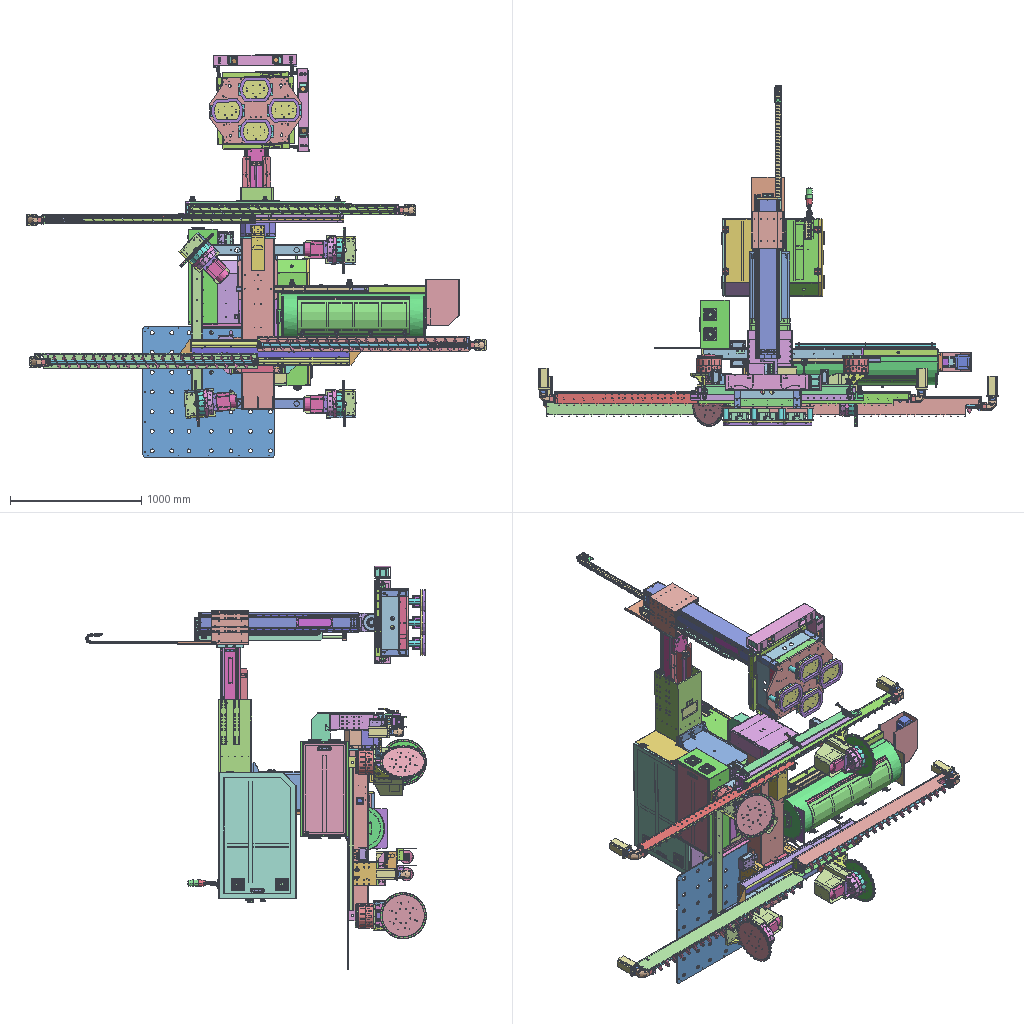Assembly | SolidWorks | 420 different items | 1007 placed | box 3503 x 2594 x 3070 mm
Parts list (item | name | quantity | parent item | size | volume | features), first 271 of 420 items:
1 | 790 Boom +300 Hydraulic Cylinder  (subassembly) | x1 | - | - | - | -
2 | (subassembly) | x4 | in 46 | 270 x 30 x 44 mm | 212143 mm3 | -
3 | (subassembly) | x4 | in 24 | 400 x 30 x 44 mm | 248543 mm3 | -
4 | (subassembly) | x4 | in 19 | 531 x 30 x 44 mm | 286413 mm3 | -
5 | (subassembly) | x2 | in 31 | - | 680804 mm3 | -
6 | (subassembly) | x1 | in 35 | 19.25 x 6.5 x 850 mm | 61984 mm3 | features AEMSimFeature 1
7 | (subassembly) | x2 | in 45 | 80.5 x 70 x 1200 mm | 2951640 mm3 | features ReferencePattern 2, LocalLPattern 1
8 | (subassembly) | x1 | - | - | - | features InContextFeatHolder 31, ReferencePattern 2, AEMSimFeature 1, CenterOfMass 1, LocalLPattern 1
9 | (subassembly) | x1 | - | - | 76260531 mm3 | features CompositeCurve 7
10 | (subassembly) | x1 | in 9 | 250.5 x 328.6 x 299.355 mm | 6826026 mm3 | -
11 | (subassembly) | x1 | in 16 | 1155 x 74 x 49 mm | 647378 mm3 | features AEMSimFeature 1
12 | (subassembly) | x1 | in 9 | 1365 x 260 x 1300 mm | 14682038 mm3 | -
13 | (subassembly) | x1 | - | 375 x 504.5 x 234 mm | 8003020 mm3 | features InContextFeatHolder 28, CompositeCurve 7
14 | (subassembly) | x4 | in 9 | 400 x 532.5 x 350 mm | 11036293 mm3 | features InContextFeatHolder 38, CompositeCurve 7
15 | (subassembly) | x1 | - | - | 69065050 mm3 | features InContextFeatHolder 16
16 | (subassembly) | x1 | - | - | 23045702 mm3 | features InContextFeatHolder 23
17 | (subassembly) | x1 | in 16 | 290 x 578 x 296 mm | 6218838 mm3 | features InContextFeatHolder 10
18 | (subassembly) | x2 | in 15, 16 | 188 x 30 x 80 mm | 347736 mm3 | features InContextFeatHolder 4
19 | (subassembly) | x1 | - | - | 22718189 mm3 | features CompositeCurve 32, InContextFeatHolder 24
20 | (subassembly) | x2 | in 19 | 630 x 120 x 80 mm | 2553807 mm3 | -
21 | (subassembly) | x4 | in 19 | 180 x 166 x 261 mm | 1533619 mm3 | features InContextFeatHolder 4
22 | (subassembly) | x1 | in 15 | 1210 x 74 x 49 mm | 674376 mm3 | features AEMSimFeature 1
23 | (subassembly) | x1 | - | - | 27603448 mm3 | features InContextFeatHolder 30, CenterOfMass 1
24 | (subassembly) | x1 | in 23 | - | 6265247 mm3 | features InContextFeatHolder 2
25 | (subassembly) | x1 | - | 312 x 120 x 1735 mm | 4939212 mm3 | features InContextFeatHolder 4
26 | (subassembly) | x1 | in 23 | 222.5 x 263.631 x 407 mm | 6113754 mm3 | features InContextFeatHolder 12
27 | (subassembly) | x4 | in 23, 49, 50 | 60 x 120 x 112 mm | 205676 mm3 | features InContextFeatHolder 4
28 | (subassembly) | x1 | - | 307 x 120 x 1730 mm | 4796774 mm3 | features InContextFeatHolder 2
29 | (subassembly) | x1 | in 31 | 286 x 85 x 1747 mm | 3475124 mm3 | features InContextFeatHolder 8, CompositeCurve 2
30 | (subassembly) | x1 | in 31 | 286 x 85 x 1747 mm | 3499831 mm3 | features InContextFeatHolder 8
31 | (subassembly) | x1 | in 23 | - | 13765877 mm3 | features InContextFeatHolder 20
32 | (subassembly) | x4 | in 41, 42 | 48 x 11 x 54 mm | 10139 mm3 | -
33 | (subassembly) | x1 | - | 645 x 163.197 x 1205 mm | 2491880 mm3 | features InContextFeatHolder 6
34 | (subassembly) | x1 | - | - | 14201492 mm3 | features InContextFeatHolder 8
35 | (subassembly) | x1 | in 34 | 487 x 297 x 1116 mm | 6337881 mm3 | features ReferencePattern 3, LocalLPattern 1
36 | (subassembly) | x1 | in 34 | 289.417 x 289.417 x 1144 mm | 3340527 mm3 | features ReferencePattern 19, CompositeCurve 2, LocalCirPattern 1
37 | (subassembly) | x1 | - | - | 11450307 mm3 | features ReferencePattern 24, InContextFeatHolder 4, LocalLPattern 3, CompositeCurve 1
38 | (subassembly) | x1 | in 37 | 730 x 365 x 229.027 mm | 2279272 mm3 | -
39 | (subassembly) | x1 | - | 1000 x 8 x 1000 mm | 7675541 mm3 | -
40 | (subassembly) | x1 | - | - | - | features InContextFeatHolder 9
41 | (subassembly) | x1 | in 40 | - | - | features InContextFeatHolder 12
42 | (subassembly) | x1 | in 40 | - | 8213820 mm3 | features InContextFeatHolder 11, ReferencePattern 7, LocalLPattern 1
43 | (subassembly) | x2 | in 15 | 648.543 x 75.872 x 50 mm | 242842 mm3 | features ReferencePattern 15, LocalLPattern 2
44 | (subassembly) | x1 | in 40 | 415.8 x 588 x 32.227 mm | 489087 mm3 | -
45 | (subassembly) | x1 | - | - | 24673962 mm3 | features InContextFeatHolder 11
46 | (subassembly) | x2 | in 45 | - | 3170015 mm3 | features InContextFeatHolder 15, CompositeCurve 2, Belt 1
47 | (subassembly) | x1 | in 45 | 120 x 307 x 1742 mm | 4964407 mm3 | features CompositeCurve 2
48 | (subassembly) | x1 | in 45 | 307 x 120 x 1742 mm | 4354852 mm3 | features CompositeCurve 2
49 | (subassembly) | x1 | - | 120 x 100 x 112 mm | 221397 mm3 | -
50 | (subassembly) | x1 | - | 178.5 x 110 x 112 mm | 250570 mm3 | -
51 | (subassembly) | x3 | in 24, 46 | 20 x 49 x 80 mm | 45972 mm3 | features AEMSimFeature 1
52 | (subassembly) | x3 | in 24, 46 | 44 x 49 x 80 mm | 74061 mm3 | features AEMSimFeature 1
53 | (subassembly) | x2 | in 16 | 960.543 x 75.872 x 50 mm | 342604 mm3 | features ReferencePattern 28, LocalLPattern 2
54 | (subassembly) | x8 | in 31, 35 | 97.135 x 31.44 x 28.2 mm | 12763 mm3 | -
55 | (subassembly) | x7 | in 9, 31 | 161.788 x 44.909 x 44.4 mm | 32694 mm3 | -
56 | (subassembly) | x1 | - | 112 x 125 x 1730 mm | 1536921 mm3 | features ReferencePattern 14, InContextFeatHolder 6, LocalLPattern 2
57 | (subassembly) | x1 | - | 127 x 125 x 1722 mm | 4062488 mm3 | -
58 | (subassembly) | x1 | - | 122 x 130 x 1720 mm | 4058025 mm3 | -
59 | (subassembly) | x1 | - | 246.625 x 216.5 x 351 mm | 5460860 mm3 | features InContextFeatHolder 2, CompositeCurve 1
60 | (subassembly) | x1 | - | 219.765 x 289 x 182 mm | 3217706 mm3 | features InContextFeatHolder 6, CompositeCurve 2
61 | (subassembly) | x1 | - | 490 x 459 x 291.379 mm | 615629 mm3 | features InContextFeatHolder 6
62 | (subassembly) | x3 | in 44 | 14.65 x 4.3 x 40 mm | 1347 mm3 | -
63 | (subassembly) | x1 | - | 150 x 131 x 2150 mm | 4854197 mm3 | -
64 | (subassembly) | x4 | in 37 | 37.408 x 96.6 x 96.6 mm | 223267 mm3 | -
65 | (subassembly) | x1 | - | 1365 x 969.6 x 1300 mm | 30670521 mm3 | features CompositeCurve 17, InContextFeatHolder 10
66 | (subassembly) | x4 | in 16 | 1215 x 30 x 44 mm | 550817 mm3 | -
67 | (subassembly) | x4 | in 15 | - | 682203 mm3 | -
68 | - | x2 | in 41 | 30 x 60 x 830 mm | 242360 mm3 | features Extrusion 1, Shell 1
69 | - | x2 | in 15 | 60 x 60 x 1234 mm | 431666 mm3 | features HoleWzd 4, Chamfer 1, Extrusion 1
70 | - | x8 | in 15, 16 | 81 x 20 x 12 mm | 16180 mm3 | features Chamfer 1, Extrusion 1, HoleWzd 1
71 | - | x1 | in 15 | 170 x 1.5 x 100 mm | 25318 mm3 | features BreakCorner 1, FlatPattern 1, HoleWzd 1, SMBaseFlange 1, SheetMetal 1
72 | - | x4 | in 15 | 20 x 220 x 35 mm | 142848 mm3 | features HoleWzd 2, Chamfer 1, Extrusion 1
73 | - | x4 | in 15 | 20 x 568 x 30 mm | 116464 mm3 | features HoleWzd 2, ICE 1, WeldMemberFeat 1, WeldmentFeature 1
74 | - | x2 | in 15 | 20 x 20 x 354 mm | 109668 mm3 | features HoleWzd 2, Chamfer 1, Extrusion 1
75 | - | x2 | in 15 | 50 x 50 x 650 mm | 247288 mm3 | features Chamfer 1, Extrusion 1, HoleWzd 1
76 | - | x1 | in 15 | 250 x 60 x 1 mm | 14915 mm3 | features BreakCorner 1, FlatPattern 1, HoleWzd 1, SMBaseFlange 1, SheetMetal 1
77 | - | x1 | in 16 | 250 x 250 x 280 mm | 2610401 mm3 | features HoleWzd 8, Chamfer 1, Cut 1, Extrusion 1, MirrorPattern 1
78 | - | x1 | in 16 | 150 x 150 x 1215 mm | 6013792 mm3 | features HoleWzd 14, ICE 3, Cut 2, Fillet 2, Extrusion 1
79 | - | x3 | in 17 | 62 x 138 x 138 mm | 462395 mm3 | features BaseBody 1
80 | - | x1 | in 16 | 84 x 70 x 50 mm | 186072 mm3 | features ICE 5, Chamfer 2, HoleWzd 2, Extrusion 1
81 | - | x4 | in 16 | 47 x 14 x 280 mm | 149226 mm3 | features HoleWzd 2, Chamfer 1, Extrusion 1, MoveFace 1
82 | - | x1 | in 16 | 70 x 278 x 1 mm | 19366 mm3 | features BreakCorner 1, FlatPattern 1, HoleWzd 1, SMBaseFlange 1, SheetMetal 1
83 | - | x2 | in 16 | 60 x 60 x 945 mm | 330466 mm3 | features HoleWzd 2, Chamfer 1, Extrusion 1
84 | - | x1 | in 16 | 257 x 300 x 20 mm | 215937 mm3 | features HoleWzd 2, BreakCorner 1, Chamfer 1, EdgeFlange 1, Extrusion 1, FlatPattern 1, SheetMetal 1, SolidToSheetMetal 1
85 | - | x1 | in 17 | 130 x 12 x 130 mm | 148815 mm3 | features HoleWzd 6, ICE 2, Chamfer 1, Cut 1, Extrusion 1
86 | - | x1 | in 17 | 130 x 12 x 130 mm | 79357 mm3 | features HoleWzd 5, Chamfer 1, Extrusion 1, ICE 1
87 | - | x1 | in 17 | 140 x 165 x 130 mm | 629581 mm3 | features HoleWzd 5, ICE 4, Chamfer 1, Extrusion 1
88 | - | x1 | in 17 | 140 x 165 x 120 mm | 582879 mm3 | features ICE 5, HoleWzd 3, Chamfer 2, Extrusion 1
89 | - | x1 | in 17 | 120 x 136 x 68 mm | 368287 mm3 | features HoleWzd 4, Chamfer 1, Extrusion 1, ICE 1
90 | - | x10 | - | 15.114 x 19.643 x 23.399 mm | 1126 mm3 | features BaseBody 1
91 | - | x1 | in 17 | 120 x 160 x 74 mm | 438042 mm3 | features HoleWzd 4, Chamfer 1, Extrusion 1, ICE 1
92 | - | x2 | in 18 | 188 x 23 x 80 mm | 151717 mm3 | features Fillet 3, HoleWzd 2, ICE 2, Chamfer 1, Extrusion 1
93 | - | x2 | in 18 | 188 x 7 x 80 mm | 69688 mm3 | features HoleWzd 2, Chamfer 1, Extrusion 1, Fillet 1
94 | - | x1 | in 19 | 700 x 15 x 500 mm | 4450228 mm3 | features HoleWzd 5, Cut 1, Extrusion 1, Fillet 1, ICE 1
95 | - | x4 | in 19 | 50 x 260 x 50 mm | 74530 mm3 | features HoleWzd 6, CirPattern 1, Extrusion 1
96 | - | x4 | in 19 | 40 x 50 x 506 mm | 247347 mm3 | features HoleWzd 4, ExtruThin 1
97 | - | x4 | in 19 | 29 x 25 x 40 mm | 10588 mm3 | features HoleWzd 2, Chamfer 1, Extrusion 1
98 | - | x2 | in 19 | 499 x 60 x 10 mm | 297280 mm3 | features HoleWzd 3, Extrusion 1
99 | - | x2 | in 19 | 479 x 60 x 10 mm | 285459 mm3 | features HoleWzd 3, Extrusion 1
100 | - | x4 | in 19 | 496 x 185 x 10 mm | 92290 mm3 | features Cut 2, HoleWzd 2, BreakCorner 1, EdgeFlange 1, FlatPattern 1, ICE 1, SMBaseFlange 1, SheetMetal 1
101 | - | x52 | - | 15.114 x 19.643 x 23.399 mm | 1126 mm3 | features BaseBody 1
102 | - | x2 | in 20 | 80 x 120 x 630 mm | 467928 mm3 | features HoleWzd 2, Cut 1, ExtruThin 1, Fillet 1, ICE 1
103 | - | x4 | in 21 | 180 x 15 x 240 mm | 528961 mm3 | features HoleWzd 4, Extrusion 1, Fillet 1, ICE 1
104 | - | x8 | in 21 | 12 x 63 x 80 mm | 50248 mm3 | features HoleWzd 7, Extrusion 1
105 | - | x4 | in 21 | 83 x 64 x 140 mm | 28826 mm3 | features HoleWzd 2, FlatPattern 1, SMBaseFlange 1, SheetMetal 1
106 | - | x4 | in 21 | 75 x 32 x 70 mm | 77130 mm3 | features HoleWzd 2, ICE 2, Extrusion 1
107 | - | x4 | in 21 | 75 x 58 x 3 mm | 8829 mm3 | features ICE 2, Extrusion 1, Fillet 1, HoleWzd 1
108 | - | x4 | in 21 | 75 x 29 x 40 mm | 38371 mm3 | features Extrusion 1, HoleWzd 1, ICE 1, MoveFace 1
109 | - | x4 | in 21 | 54.631 x 35.5 x 20 mm | 24661 mm3 | features ICE 3, Extrusion 1, Fillet 1, HoleWzd 1
110 | - | x2 | in 23 | 40 x 80 x 60 mm | 12649 mm3 | features HoleWzd 2, BreakCorner 1, FlatPattern 1, SMBaseFlange 1, SheetMetal 1
111 | - | x1 | in 24 | 250 x 400 x 100 mm | 1758243 mm3 | features HoleWzd 10, Fillet 3, ICE 3, Cut 2, Extrusion 1, MirrorPattern 1
112 | - | x1 | in 24 | 60 x 135 x 60 mm | 337667 mm3 | features BaseBody 1
113 | - | x1 | in 24 | 12 x 345 x 110 mm | 373766 mm3 | features HoleWzd 4, Cut 1, Extrusion 1
114 | - | x1 | in 24 | 12 x 345 x 110 mm | 373766 mm3 | features HoleWzd 4, Cut 1, Extrusion 1
115 | - | x1 | in 24 | 10 x 330 x 180 mm | 549177 mm3 | features Cut 2, HoleWzd 2, Chamfer 1, Extrusion 1, MoveFace 1
116 | - | x1 | in 24 | 55 x 65.5 x 30 mm | 74891 mm3 | features HoleWzd 3, Chamfer 2, ICE 2, Extrusion 1
117 | - | x4 | in 24 | 35 x 12 x 16 mm | 5336 mm3 | features Chamfer 1, Extrusion 1, HoleWzd 1
118 | - | x1 | in 24 | 100 x 60 x 110 mm | 155366 mm3 | features Chamfer 2, HoleWzd 2, Extrusion 1, MoveFace 1
119 | - | x1 | in 24 | 347 x 403 x 127.5 mm | 464397 mm3 | features HoleWzd 3, ICE 3, Cut 2, FlatPattern 2, SheetMetal 2, SolidToSheetMetal 2, BreakCorner 1, Chamfer 1, EdgeFlange 1, Extrusion 1, MirrorPattern 1
120 | - | x1 | in 24 | 260 x 145 x 128 mm | 125858 mm3 | features Chamfer 2, EdgeFlange 2, Extrusion 1, FlatPattern 1, HoleWzd 1, SheetMetal 1, SolidToSheetMetal 1
121 | - | x1 | in 24 | 250 x 1.5 x 100 mm | 37100 mm3 | features BreakCorner 1, FlatPattern 1, HoleWzd 1, ICE 1, SMBaseFlange 1, SheetMetal 1
122 | - | x1 | in 24 | 104 x 10 x 60 mm | 39122 mm3 | features HoleWzd 4, Cut 2, Chamfer 1, Extrusion 1
123 | - | x2 | in 34 | 55 x 55 x 13 mm | 21668 mm3 | features Extrusion 1, Fillet 1
124 | - | x1 | in 24 | 70 x 10 x 60 mm | 36663 mm3 | features HoleWzd 4, Chamfer 1, Extrusion 1
125 | - | x2 | in 24 | 40 x 30 x 8 mm | 6006 mm3 | features Chamfer 1, Extrusion 1, HoleWzd 1
126 | - | x1 | in 24 | 100 x 60 x 110 mm | 155366 mm3 | features Chamfer 2, HoleWzd 2, Extrusion 1, MoveFace 1
127 | - | x1 | - | 120 x 75 x 1000 mm | 1739267 mm3 | features HoleWzd 5, Cut 2, MoveFace 2, Chamfer 1, Extrusion 1, Fillet 1
128 | - | x2 | in 47, 48 | 100 x 100 x 1604 mm | 874347 mm3 | features MoveFace 6, ICE 2, BaseBody 1, Helix 1, Sweep 1
129 | - | x2 | in 47, 48 | 50 x 50 x 10 mm | 11856 mm3 | features ICE 2, Chamfer 1, Extrusion 1, HoleWzd 1
130 | - | x4 | in 29, 30, 47, 48 | 50 x 50 x 10 mm | 10238 mm3 | features ICE 2, Chamfer 1, Extrusion 1, HoleWzd 1
131 | - | x4 | in 29, 30, 47, 48 | 62 x 62 x 12 mm | 24839 mm3 | features ICE 3, HoleWzd 2, Chamfer 1, Extrusion 1
132 | - | x1 | in 47 | 92 x 99 x 15 mm | 82233 mm3 | features MirrorStock 1
133 | - | x1 | in 47 | 87 x 94 x 12 mm | 62817 mm3 | features MirrorStock 1
134 | - | x10 | in 15, 16, 17, 26, 29, 30, 47, 48 | 180 x 81 x 81 mm | 861564 mm3 | features BaseBody 1, MoveFace 1
135 | - | x4 | in 29, 30, 47, 48 | 85 x 13 x 85 mm | 56434 mm3 | features ICE 3, HoleWzd 2, Chamfer 1, Extrusion 1
136 | - | x1 | - | 150 x 120 x 1609 mm | 2357171 mm3 | features HoleWzd 7, Fillet 2, Cut 1, Extrusion 1, ICE 1, LPattern 1, MoveFace 1
137 | - | x1 | in 48 | 87 x 94 x 12 mm | 62817 mm3 | features HoleWzd 4, Cut 2, MoveFace 2, Chamfer 1, Extrusion 1, Fillet 1, ICE 1
138 | - | x1 | in 48 | 92 x 99 x 15 mm | 82233 mm3 | features HoleWzd 4, Cut 2, MoveFace 2, Chamfer 1, Extrusion 1, Fillet 1, ICE 1, MoveCopyBody 1
139 | - | x1 | in 26 | 260 x 260 x 20 mm | 876981 mm3 | features HoleWzd 6, Chamfer 3, ICE 2, Extrusion 1, Fillet 1
140 | - | x1 | in 26 | 100 x 17.5 x 100 mm | 79036 mm3 | features ICE 6, HoleWzd 4, Chamfer 3, Extrusion 1, Fillet 1
141 | - | x1 | in 26 | 262.631 x 60 x 222.5 mm | 1391855 mm3 | features HoleWzd 5, ICE 5, Chamfer 1, Cut 1, Fillet 1, Revolution 1
142 | - | x1 | in 26 | 44 x 47.656 x 48 mm | 38750 mm3 | features ICE 5, HoleWzd 4, BaseBody 1, Chamfer 1, RevCut 1
143 | - | x1 | in 26 | 263 x 130.5 x 136 mm | 76891 mm3 | features HoleWzd 2, Chamfer 1, Cut 1, Extrusion 1, Shell 1
144 | - | x1 | in 26 | 263 x 130.5 x 136 mm | 68260 mm3 | features Cut 2, HoleWzd 2, Chamfer 1, Extrusion 1, Shell 1
145 | - | x1 | in 41 | 110 x 15 x 20 mm | 32457 mm3 | features Extrusion 1, HoleWzd 1
146 | - | x1 | in 26 | 340 x 95 x 103 mm | 87299 mm3 | features EdgeFlange 1, Extrusion 1, FlatPattern 1, HoleWzd 1, ICE 1, SheetMetal 1, SolidToSheetMetal 1
147 | - | x4 | in 27 | 60 x 120 x 90 mm | 122991 mm3 | features HoleWzd 4, Extrusion 1, Shell 1
148 | - | x4 | in 27 | 60 x 120 x 4 mm | 27931 mm3 | features Extrusion 1, HoleWzd 1, ICE 1
149 | - | x4 | in 27 | 60 x 120 x 4 mm | 16436 mm3 | features HoleWzd 4, ICE 3, Extrusion 1, Fillet 1
150 | - | x4 | in 27 | 50 x 110 x 2 mm | 11000 mm3 | features Extrusion 1
151 | - | x1 | in 31 | 150 x 105 x 1200 mm | 2927452 mm3 | features HoleWzd 7, Extrusion 1, MoveFace 1
152 | - | x1 | in 31 | 120 x 75 x 1150 mm | 2118632 mm3 | features HoleWzd 4, Extrusion 1
153 | - | x2 | in 31 | 70 x 50 x 60 mm | 59657 mm3 | features HoleWzd 2, Chamfer 1, Extrusion 1
154 | - | x1 | in 31 | 80 x 99 x 60 mm | 93057 mm3 | features HoleWzd 2, Chamfer 1, Extrusion 1
155 | - | x1 | in 31 | 80 x 22 x 60 mm | 46558 mm3 | features HoleWzd 2, Chamfer 1, Extrusion 1
156 | - | x2 | in 15, 16 | 90.001 x 150.5 x 90.001 mm | 719392 mm3 | features BaseBody 1
157 | - | x1 | in 30 | 110 x 70 x 1620 mm | 1292912 mm3 | features HoleWzd 8, Extrusion 1, Fillet 1, ICE 1, LPattern 1
158 | - | x2 | in 29, 30 | 60 x 60 x 1608 mm | 669681 mm3 | features MoveFace 7, ICE 2, BaseBody 1, Helix 1, Sweep 1
159 | - | x2 | in 29, 30 | 50 x 50 x 10 mm | 15222 mm3 | features ICE 2, Chamfer 1, Extrusion 1, HoleWzd 1
160 | - | x1 | in 30 | 65 x 81 x 15 mm | 49071 mm3 | features HoleWzd 2, MoveFace 2, MirrorStock 1
161 | - | x1 | in 30 | 60 x 76 x 12 mm | 39739 mm3 | features HoleWzd 2, MoveFace 2, MirrorStock 1
162 | - | x1 | in 29 | 110 x 70 x 1620 mm | 1267846 mm3 | features HoleWzd 8, MoveFace 3, Fillet 2, LPattern 2, Cut 1, Extrusion 1, ICE 1
163 | - | x1 | in 29 | 65 x 81 x 15 mm | 49071 mm3 | features HoleWzd 4, Cut 2, MoveFace 2, Chamfer 1, Extrusion 1, Fillet 1, ICE 1, MoveCopyBody 1
164 | - | x1 | in 29 | 60 x 76 x 12 mm | 39739 mm3 | features HoleWzd 4, MoveFace 3, Cut 2, Chamfer 1, Extrusion 1, Fillet 1, ICE 1
165 | - | x1 | in 34 | 142 x 173 x 34 mm | 50656 mm3 | features EdgeFlange 2, HoleWzd 2, BreakCorner 1, FlatPattern 1, MoveFace 1, SMBaseFlange 1, SheetMetal 1
166 | - | x8 | in 41, 42, 64 | 92 x 92.001 x 25.408 mm | 167387 mm3 | features BaseBody 1
167 | - | x1 | in 34 | 187 x 372 x 254 mm | 400780 mm3 | features FlatPattern 2, SheetMetal 2, BreakCorner 1, Chamfer 1, Extrusion 1, HoleWzd 1, SMBaseFlange 1, SolidToSheetMetal 1
168 | - | x1 | in 34 | 110 x 110 x 16 mm | 113885 mm3 | features ICE 3, Chamfer 2, HoleWzd 2, Extrusion 1
169 | - | x1 | in 34 | 100 x 100 x 15 mm | 98385 mm3 | features HoleWzd 2, ICE 2, Chamfer 1, Extrusion 1
170 | - | x1 | in 34 | 140 x 140 x 24 mm | 366967 mm3 | features HoleWzd 3, ICE 3, Chamfer 1, Cut 1, Extrusion 1
171 | - | x1 | in 35 | 487 x 297 x 1116 mm | 5128142 mm3 | features ICE 12, HoleWzd 7, Fillet 4, MoveCopyBody 4, Chamfer 3, LPattern 3, Stock 3, Cut 1, Extrusion 1, Shell 1
172 | - | x1 | in 35 | 284.209 x 71.481 x 850 mm | 1096694 mm3 | features ExtruThin 1, ICE 1
173 | - | x1 | in 36 | 60 x 60 x 92 mm | 149406 mm3 | features ICE 6, Chamfer 1, Extrusion 1, HoleWzd 1
174 | - | x1 | in 36 | 291 x 291 x 5 mm | 156823 mm3 | features ICE 2, Extrusion 1, Fillet 1
175 | - | x2 | in 36 | 291 x 291 x 5 mm | 163158 mm3 | features ICE 2, Extrusion 1, Fillet 1
176 | - | x1 | in 36 | 1022 x 30 x 30 mm | 722056 mm3 | features ICE 3, WeldMemberFeat 1, WeldmentFeature 1
177 | - | x8 | in 14 | 65 x 65 x 7 mm | 9271 mm3 | features BaseBody 1
178 | - | x1 | in 36 | 60 x 60 x 90 mm | 128146 mm3 | features ICE 8, HoleWzd 2, Chamfer 1, Extrusion 1
179 | - | x20 | in 36 | 1072 x 25 x 3 mm | 80400 mm3 | features FlatPattern 1, SMBaseFlange 1, SheetMetal 1
180 | - | x1 | in 36 | 181 x 462.5 x 181 mm | 124893 mm3 | features Helix 1, Sweep 1
181 | - | x1 | in 36 | 181 x 462.5 x 181 mm | 124893 mm3 | features Helix 1, Sweep 1
182 | - | x1 | in 38 | 730 x 365 x 221.5 mm | 1200734 mm3 | features HoleWzd 6, ICE 4, EdgeFlange 3, FlatPattern 1, SheetMetal 1, SolidToSheetMetal 1
183 | - | x1 | in 38 | 693 x 342.263 x 15 mm | 608896 mm3 | features EdgeFlange 3, FlatPattern 2, ICE 2, MoveCopyBody 2, SMBaseFlange 2, SheetMetal 2, Chamfer 1, Cut 1, HoleWzd 1, Stock 1
184 | - | x1 | in 38 | 660 x 305 x 12 mm | 436518 mm3 | features HoleWzd 2, EdgeFlange 1, FlatPattern 1, SMBaseFlange 1, SheetMetal 1
185 | - | x1 | in 39 | 1000 x 8 x 1000 mm | 7675541 mm3 | features HoleWzd 2, MoveFace 2, Cut 1, Extrusion 1, Fillet 1, ICE 1, LPattern 1
186 | - | x2 | in 40 | 20 x 90.5 x 416.5 mm | 94970 mm3 | features EdgeFlange 2, FlatPattern 1, HoleWzd 1, ICE 1, SMBaseFlange 1, SheetMetal 1
187 | - | x1 | in 40 | 298 x 21.5 x 551.5 mm | 305724 mm3 | features EdgeFlange 2, Cut 1, FlatPattern 1, HoleWzd 1, SMBaseFlange 1, SheetMetal 1
188 | - | x4 | in 29, 30, 47, 48 | 35 x 35 x 10 mm | 5588 mm3 | features BaseBody 1
189 | - | x1 | in 40 | 20 x 140 x 90 mm | 21403 mm3 | features HoleWzd 2, BreakCorner 1, FlatPattern 1, SMBaseFlange 1, SheetMetal 1
190 | - | x1 | in 41 | 264.5 x 588 x 960 mm | 1725944 mm3 | features HoleWzd 16, ICE 8, Cut 6, FlatPattern 6, SheetMetal 6, SolidToSheetMetal 4, SMBaseFlange 3, EdgeFlange 2, MoveFace 2, Chamfer 1, Extrusion 1
191 | - | x1 | in 41 | 959 x 587 x 21.5 mm | 1078977 mm3 | features EdgeFlange 4, FlatPattern 4, SMBaseFlange 4, SheetMetal 4, HoleWzd 3, Cut 2, ICE 1
192 | - | x1 | in 41 | 830 x 530 x 15 mm | 919562 mm3 | features HoleWzd 2, BreakCorner 1, Cut 1, EdgeFlange 1, FlatPattern 1, SMBaseFlange 1, SheetMetal 1
193 | - | x1 | in 42 | 233 x 588 x 960 mm | 1652161 mm3 | features HoleWzd 15, FlatPattern 7, ICE 7, SheetMetal 7, SolidToSheetMetal 6, Cut 5, EdgeFlange 3, Chamfer 1, Extrusion 1, SMBaseFlange 1
194 | - | x1 | in 42 | 959 x 587 x 21.5 mm | 1078977 mm3 | features MirrorStock 1
195 | - | x1 | in 42 | 830 x 530 x 15 mm | 919972 mm3 | features HoleWzd 1, ICE 1, MirrorStock 1
196 | - | x1 | in 44 | 16 x 588 x 411.5 mm | 451920 mm3 | features EdgeFlange 2, Cut 1, FlatPattern 1, HoleWzd 1, SMBaseFlange 1, SheetMetal 1
197 | - | x2 | in 45 | 120 x 86 x 195 mm | 136249 mm3 | features HoleWzd 2, BreakCorner 1, Cut 1, EdgeFlange 1, ExtruThin 1, FlatPattern 1, SheetMetal 1, SolidToSheetMetal 1
198 | - | x1 | in 45 | 1200 x 80 x 25 mm | 115619 mm3 | features MoveFace 2, BreakCorner 1, Cut 1, EdgeFlange 1, FlatPattern 1, HoleWzd 1, SMBaseFlange 1, SheetMetal 1
199 | - | x4 | in 29, 30, 47, 48 | 47 x 47 x 12 mm | 12629 mm3 | features BaseBody 1
200 | - | x1 | in 45 | 1200 x 80 x 25 mm | 115619 mm3 | features MirrorStock 1
201 | - | x2 | in 45 | 249 x 116 x 90 mm | 48716 mm3 | features EdgeFlange 2, BreakCorner 1, FlatPattern 1, HoleWzd 1, ICE 1, MoveFace 1, SMBaseFlange 1, SheetMetal 1
202 | - | x1 | in 45 | 195 x 12 x 1200 mm | 2789805 mm3 | features HoleWzd 6, Extrusion 1, ICE 1
203 | - | x1 | in 45 | 90 x 60 x 255 mm | 315166 mm3 | features Chamfer 3, HoleWzd 2, ExtruThin 1
204 | - | x1 | in 45 | 90 x 60 x 255 mm | 315166 mm3 | features MirrorStock 1
205 | - | x2 | in 46 | 180 x 270 x 36 mm | 970158 mm3 | features HoleWzd 11, ICE 2, Cut 1, Extrusion 1, Fillet 1
206 | - | x2 | in 46 | 75 x 39.5 x 34 mm | 65045 mm3 | features HoleWzd 3, Chamfer 2, ICE 2, Extrusion 1
207 | - | x2 | in 46 | 175 x 275 x 15 mm | 588428 mm3 | features HoleWzd 4, Extrusion 1, ICE 1
208 | - | x2 | in 46 | 160 x 8 x 82 mm | 66317 mm3 | features HoleWzd 2, Extrusion 1, Fillet 1, ICE 1
209 | - | x2 | in 46 | 105 x 30 x 120 mm | 37376 mm3 | features HoleWzd 2, BreakCorner 1, Cut 1, Extrusion 1, FlatPattern 1, ICE 1, SheetMetal 1, SolidToSheetMetal 1
210 | - | x2 | in 46 | 184 x 270 x 86 mm | 96917 mm3 | features HoleWzd 2, Extrusion 1, ICE 1, Shell 1
211 | - | x1 | in 47 | 150 x 120 x 1700 mm | 2499600 mm3 | features HoleWzd 10, Fillet 2, LPattern 2, Cut 1, Extrusion 1, ICE 1, MoveFace 1
212 | - | x1 | in 48 | 150 x 120 x 1609 mm | 2345426 mm3 | features HoleWzd 7, Fillet 2, LPattern 2, Cut 1, Extrusion 1, ICE 1, MoveFace 1
213 | - | x4 | in 29, 47, 48 | 50 x 50 x 6 mm | 13563 mm3 | features ICE 3, Chamfer 1, Extrusion 1, HoleWzd 1
214 | - | x1 | in 49 | 40 x 80 x 60 mm | 15721 mm3 | features HoleWzd 2, BreakCorner 1, FlatPattern 1, SMBaseFlange 1, SheetMetal 1
215 | - | x1 | in 50 | 50 x 170 x 70 mm | 44894 mm3 | features HoleWzd 2, BreakCorner 1, FlatPattern 1, Gusset 1, SMBaseFlange 1, SheetMetal 1
216 | - | x2 | in 46 | 46.2 x 152.2 x 15 mm | 20675 mm3 | features BeltProfileFeature 1, ExtruThin 1
217 | - | x1 | in 10 | 250.5 x 250.5 x 122.6 mm | 3466893 mm3 | features BaseBody 1
218 | - | x2 | in 15, 16 | 26 x 60 x 88 mm | 94371 mm3 | features BaseBody 3
219 | - | x4 | in 20 | 196.4 x 105.4 x 59 mm | 1042939 mm3 | features BaseBody 3
220 | - | x2 | in 46 | 21 x 44 x 44 mm | 20059 mm3 | features BaseBody 1
221 | - | x2 | in 46 | 21 x 44 x 44 mm | 16333 mm3 | features BaseBody 1
222 | - | x1 | in 19 | 146.9 x 109.2 x 38 mm | 517225 mm3 | features BaseBody 9
223 | - | x4 | in 14 | 130 x 170 x 202 mm | 1970646 mm3 | features ICE 11, Chamfer 2, Fillet 2, HoleWzd 2, Extrusion 1
224 | - | x3 | in 37 | 50 x 210 x 100 mm | 965694 mm3 | features HoleWzd 2, Extrusion 1, ICE 1
225 | - | x6 | in 14, 46 | 92.5 x 148 x 80 mm | 645645 mm3 | features BaseBody 6
226 | - | x2 | in 15, 16 | 69 x 60 x 88 mm | 168819 mm3 | features BaseBody 9
227 | - | x4 | in 38, 41, 42, 44 | 59.2 x 32.227 x 110 mm | 33125 mm3 | features BaseBody 1
228 | - | x1 | in 19 | 145 x 40 x 90 mm | 467276 mm3 | features Extrusion 1, HoleWzd 1, ICE 1
229 | - | x1 | in 41 | 65 x 79.307 x 65.435 mm | 93271 mm3 | features BaseBody 13
230 | - | x1 | in 41 | - | - | features BaseBody 25, RefSurface 9
231 | - | x1 | in 41 | 70 x 236.301 x 70 mm | 289384 mm3 | features BaseBody 9
232 | - | x8 | in 41, 42, 64 | 96.6 x 96.6 x 10.5 mm | 55881 mm3 | features BaseBody 3
233 | - | x1 | in 41 | 45 x 64 x 90 mm | 259200 mm3 | features Extrusion 1
234 | - | x5 | in 24, 29, 30, 47, 48 | 105 x 143.9 x 60 mm | 435944 mm3 | features BaseBody 10
235 | - | x1 | in 34 | 247 x 90 x 141 mm | 1704334 mm3 | features BaseBody 30
236 | - | x1 | in 26 | 85 x 85 x 145.3 mm | 617481 mm3 | features BaseBody 3
237 | - | x1 | in 41 | - | 778602 mm3 | features BaseBody 96
238 | - | x4 | in 46 | 49 x 11.547 x 10 mm | 1608 mm3 | features RevCut 3, Boss 1, Chamfer 1, Extrusion 1, Fillet 1, LPattern 1
239 | - | x4 | in 46 | 11.547 x 10 x 6.4 mm | 424.571 mm3 | features RevCut 2, Extrusion 1, LPattern 1
240 | - | x1 | in 19 | 70 x 23 x 118 mm | 188768 mm3 | features Extrusion 1, Fillet 1, HoleWzd 1
241 | - | x6 | in 14, 34, 45 | 14.4 x 14 x 14 mm | 897.239 mm3 | features Cut 2, RevCut 2, Boss 1, Extrusion 1, Fillet 1, LPattern 1
242 | - | x8 | in 14, 45, 46 | 51 x 10 x 10 mm | 1665 mm3 | features Fillet 2, RevCut 2, Boss 1, Chamfer 1, Cut 1, Extrusion 1, LPattern 1
243 | - | x1 | in 19 | 64 x 23 x 45 mm | 65028 mm3 | features Extrusion 1, Fillet 1, HoleWzd 1
244 | - | x1 | in 10 | 100 x 10 x 100 mm | 28032 mm3 | features Extrusion 1, Fillet 1
245 | - | x12 | in 18 | 44 x 7 x 44 mm | 4885 mm3 | features Extrusion 1, ICE 1
246 | - | x1 | - | 70 x 200 x 120 mm | 169957 mm3 | features HoleWzd 2, Cut 1, Extrusion 1, ICE 1
247 | - | x8 | in 21 | 88 x 131 x 55 mm | 138232 mm3 | features ICE 2, Extrusion 1, HoleWzd 1
248 | - | x1 | in 24 | 66 x 40 x 40 mm | 67909 mm3 | features BaseBody 3
249 | - | x4 | in 21 | 180 x 20 x 240 mm | 299340 mm3 | features Extrusion 1, Fillet 1
250 | - | x1 | in 41 | 170 x 40 x 180 mm | 1224000 mm3 | features Extrusion 1
251 | - | x1 | - | 60 x 60 x 60 mm | 25462 mm3 | features HoleWzd 2, Chamfer 1, Extrusion 1
252 | - | x1 | - | 70 x 200 x 120 mm | 169957 mm3 | features HoleWzd 2, Cut 1, Extrusion 1, ICE 1
253 | - | x1 | - | 80 x 125 x 1600 mm | 2537389 mm3 | features HoleWzd 8, Extrusion 1, Fillet 1
254 | - | x1 | - | 610 x 105 x 25 mm | 182488 mm3 | features ICE 2, BreakCorner 1, EdgeFlange 1, FlatPattern 1, HoleWzd 1, LPattern 1, SMBaseFlange 1, SheetMetal 1
255 | - | x1 | - | 1600 x 105 x 3 mm | 430207 mm3 | features FlatPattern 1, HoleWzd 1, ICE 1, LPattern 1, SMBaseFlange 1, SheetMetal 1
256 | - | x1 | - | 235 x 262.5 x 23 mm | 355148 mm3 | features ICE 2, Cut 1, Extrusion 1, HoleWzd 1
257 | - | x2 | in 37 | 125 x 40 x 5 mm | 23157 mm3 | features Extrusion 1, Fillet 1
258 | - | x11 | in 19, 41, 42 | 175 x 98 x 33 mm | 507848 mm3 | features BaseBody 1
259 | - | x4 | in 18 | 28 x 56.856 x 56.856 mm | 33698 mm3 | features ICE 3, BaseBody 1
260 | - | x2 | in 18 | 28 x 56.856 x 56.856 mm | 29625 mm3 | features ICE 4, BaseBody 1
261 | - | x4 | in 29, 30, 47, 48 | 40 x 40 x 8 mm | 7526 mm3 | features Extrusion 1, Fillet 1
262 | - | x4 | in 29, 30, 47, 48 | 40 x 40 x 7 mm | 4473 mm3 | features Extrusion 1, Fillet 1
263 | - | x2 | in 34 | 60 x 60 x 8 mm | 14794 mm3 | features Extrusion 1, Fillet 1
264 | - | x1 | - | 310 x 100 x 650 mm | 20150000 mm3 | features Extrusion 1
265 | - | x4 | in 27 | 40 x 80 x 1 mm | 3200 mm3 | features Extrusion 1
266 | - | x1 | - | 110 x 120 x 60 mm | 791822 mm3 | features Extrusion 1, HoleWzd 1, PLine 1
267 | - | x1 | in 37 | 692 x 342 x 2 mm | 60240 mm3 | features Extrusion 1
268 | - | x1 | in 16 | 35 x 175 x 100 mm | 562241 mm3 | features HoleWzd 2, ICE 2, Extrusion 1
269 | - | x1 | in 15 | 300 x 210 x 600 mm | 37800000 mm3 | features Extrusion 1
270 | - | x1 | in 41 | 180 x 60 x 60 mm | 644743 mm3 | features Extrusion 1, HoleWzd 1
271 | - | x1 | in 19 | 90 x 23 x 30 mm | 60888 mm3 | features Extrusion 1, Fillet 1, HoleWzd 1
Mates (type | each side: item.copy, entity, surface, feature), first 280 of 1373 lines:
In the top assembly
Coincident | 77.1 face plane Boss-Extrude 1 | 391.1 face plane Boss-Extrude 1
Width | 77.1 face plane Boss-Extrude 1 | 77.1 face plane Boss-Extrude 1 | 391.1 face plane Boss-Extrude 1 | 391.1 face plane Boss-Extrude 1 | 2 times
Width | assembly face | assembly face | assembly face | assembly face | 14 times
Coincident | assembly face | assembly face | 10 times
DistanceDim | assembly face | assembly face | 2 times
Coincident | assembly face | 182.1 face plane  Convert Body 1 | 2 times
Width | assembly face | assembly face | assembly face
Parallel | assembly face | assembly face | 3 times
Coincident | assembly face | 185.1 face plane Boss-Extrude 1 | 2 times
Coincident | 389.1 face plane Boss-Extrude 1 | 357.1 face plane Boss-Extrude 1
Width | 357.1 face plane  Square Tube 300 X 300 X 8.0(1) | 357.1 face plane  Square Tube 300 X 300 X 8.0(1) | 389.1 face plane Boss-Extrude 1 | 389.1 face plane Boss-Extrude 1
Width | 389.1 face plane Boss-Extrude 1 | 389.1 face plane Boss-Extrude 1 | 357.1 face plane  Square Tube 300 X 300 X 8.0(1) | 357.1 face plane  Square Tube 300 X 300 X 8.0(1)
Coincident | 389.1 face plane Boss-Extrude 1 | 193.1 face plane  Convert Body 4
Coincident | 389.1 face plane Boss-Extrude 1 | 193.1 face plane  Convert Body 1
Coincident | 357.1 face plane  Square Tube 300 X 300 X 8.0(1) | 193.1 face plane  Convert Body 1
Coincident | 389.1 face plane Boss-Extrude 1 | 190.1 face plane  Convert Body 9
Coincident | 389.1 face plane Boss-Extrude 1 | 190.1 face plane  Convert Body 10
Coincident | 357.1 face plane  Square Tube 300 X 300 X 8.0(1) | 190.1 face plane  Convert Body 9
Parallel | assembly face | 389.1 face plane Boss-Extrude 1
DistanceDim | 182.1 face plane  Convert Body 1 | 185.1 face plane Boss-Extrude 1
Coincident | 91.1 face plane Boss-Extrude 1 | 94.1 face plane Boss-Extrude 1
DistanceDim | 91.1 face plane Boss-Extrude 1 | 94.1 face plane Boss-Extrude 1
Width | 94.1 face plane Boss-Extrude 1 | 94.1 face plane Boss-Extrude 1 | 91.1 face plane Boss-Extrude 1 | 91.1 face plane Boss-Extrude 1
Coincident | assembly face | 139.1 face plane Boss-Extrude 1 | 2 times
Width | 139.1 face plane Boss-Extrude 1 | 139.1 face plane Boss-Extrude 1 | assembly face | assembly face
DistanceDim | assembly face | 185.1 face plane Boss-Extrude 1
Coincident | assembly face | 148.1 face plane Boss-Extrude 1
Coincident | assembly face | 147.1 face plane Boss-Extrude 1
Coincident | assembly face | 171.1 face plane Boss-Extrude 3 | 2 times
Coincident | assembly face | 171.1 face plane Boss-Extrude 2
DistanceDim | 165.1 face plane Base-Flange 1 | assembly face
Width | assembly face | assembly face | 205.1 face plane Boss-Extrude 1 | 205.2 face plane Boss-Extrude 1
Coincident | 103.1 face plane Boss-Extrude 1 | assembly face
DistanceDim | assembly face | 205.2 face plane Boss-Extrude 1
DistanceDim | 147.1 face plane Boss-Extrude 1 | assembly face
DistanceDim | 182.1 face plane  Convert Body 1 | 147.1 face plane Boss-Extrude 1
Coincident | 147.1 face plane Boss-Extrude 1 | 147.2 face plane Boss-Extrude 1
DistanceDim | 205.1 face plane Boss-Extrude 1 | assembly face
DistanceDim | 148.2 face plane Boss-Extrude 1 | 210.1 face plane Boss-Extrude 1
Coincident | assembly face | 147.2 face plane Boss-Extrude 1
DistanceDim | 171.1 face plane Boss-Extrude 3 | assembly face
DistanceDim | 185.1 face plane Boss-Extrude 1 | assembly face
Coincident | 365.1 face plane Boss-Extrude 1 | 139.1 face plane Boss-Extrude 1 | 2 times
Width | 365.1 face plane Boss-Extrude 1 | 365.1 face plane Boss-Extrude 1 | 139.1 face plane Boss-Extrude 1 | 139.1 face plane Boss-Extrude 1
Coincident | 366.1 face plane Gb/6728-1986 Square Hollow Section 050 X 50 X 4(1) | 171.1 face plane Boss-Extrude 3
Width | 366.2 face plane Gb/6728-1986 Square Hollow Section 050 X 50 X 4(1) | 366.1 face plane Gb/6728-1986 Square Hollow Section 050 X 50 X 4(1) | 171.1 face plane Boss-Extrude 3 | 171.1 face plane Boss-Extrude 3
DistanceDim | 171.1 face plane Boss-Extrude 1 | 350.1 face plane Boss-Extrude 2
Coincident | 352.1 face plane Boss-Extrude 1 | 182.1 face plane  Convert Body 1
DistanceDim | 182.1 face plane Edge-Flange 1 | 352.1 face plane Boss-Extrude 4
DistanceDim | 182.1 face plane  Convert Body 1 | 352.1 face plane Boss-Extrude 1
Coincident | 350.1 face plane Boss-Extrude 2 | 185.1 face plane Boss-Extrude 1
Coincident | 350.1 face plane Boss-Extrude 5 | 185.1 face plane Boss-Extrude 1
DistanceDim | 350.1 face plane Boss-Extrude 5 | 205.1 face plane Boss-Extrude 1
DistanceDim | 205.1 face plane Boss-Extrude 1 | 351.1 face plane Boss-Extrude 1
Coincident | 350.1 face plane Boss-Extrude 3 | 205.1 face plane Boss-Extrude 1
DistanceDim | 215.1 face plane Base-Flange 1 | 350.1 face plane Boss-Extrude 5
Coincident | 352.1 face plane Boss-Extrude 1 | 214.1 face plane Base-Flange 1
Coincident | 352.1 face plane Boss-Extrude 1 | 147.1 face plane Boss-Extrude 1
In subassembly 9
Concentric | 353.1 edge | 354.1 edge
Coincident | 353.1 face plane Boss-Extrude 1 | 354.1 face plane Boss-Extrude 1
Coincident | 354.1 face plane Boss-Extrude 1 | 217.1 face plane  Import 1
Concentric | 354.1 face cylinder Boss-Extrude 1 | 370.1 face cylinder Revolve 1
Concentric | 353.1 face cylinder M52 Clearance Hole 1 | 354.1 face cylinder Boss-Extrude 1
Width | 357.2 face plane  Square Tube 300 X 300 X 8.0(1) | 357.2 face plane  Square Tube 300 X 300 X 8.0(1) | 370.1 face plane Boss-Extrude 1 | 370.1 face plane Boss-Extrude 1
Concentric | 357.2 face cylinder Cut-Extrude 5 | 217.1 face cylinder  Import 1
Concentric | 357.2 face cylinder M10 Clearance Hole 2 | 242.1 face
Coincident | 357.2 face plane Boss-Extrude 4 | 242.1 face
Coincident | assembly face | assembly face
Concentric | assembly face | assembly face | 2 times
Coincident | 357.2 face plane  Square Tube 300 X 300 X 8.0(1) | 362.1 face plane Edge-Flange 2
Width | 357.2 face plane  Square Tube 300 X 300 X 8.0(1) | 357.2 face plane  Square Tube 300 X 300 X 8.0(1) | 362.1 face plane Edge-Flange 1 | 362.1 face plane Edge-Flange 1
Coincident | 357.2 face plane Boss-Extrude 4 | 370.1 face plane Revolve 1
Width | 364.1 face plane Boss-Extrude 1 | 364.1 face plane Boss-Extrude 1 | 357.2 face plane  Square Tube 300 X 300 X 8.0(1) | 357.2 face plane  Square Tube 300 X 300 X 8.0(1)
DistanceDim | 357.2 face plane  Square Tube 300 X 300 X 8.0(1) | 364.1 face plane Boss-Extrude 1
DistanceDim | 357.2 face plane Boss-Extrude 4 | 364.1 face plane Boss-Extrude 1
Width | 363.1 face plane Boss-Extrude 1 | 363.1 face plane Boss-Extrude 1 | 357.2 face plane  Square Tube 300 X 300 X 8.0(1) | 357.2 face plane  Square Tube 300 X 300 X 8.0(1)
Coincident | 364.1 face plane Boss-Extrude 1 | 363.1 face plane Boss-Extrude 1
Coincident | 357.2 face plane  Square Tube 300 X 300 X 8.0(1) | 363.1 face plane  Shell 1
Coincident | 362.1 face plane Base-Flange 1 | 363.1 face plane Boss-Extrude 1
Coincident | 367.1 face plane Gb/6728-1986 Square Hollow Section 040 X 40 X 4(1) | 367.2 face plane Gb/6728-1986 Square Hollow Section 040 X 40 X 4(1)
Parallel | 350.2 face plane Boss-Extrude 3 | 9.1 plane
Coincident | 350.2 face plane Boss-Extrude 4 | 358.1 face plane Base-Flange 1
Width | 350.2 face plane Boss-Extrude 3 | 350.2 face plane Boss-Extrude 2 | 358.1 face plane Base-Flange 1 | 358.1 face plane Base-Flange 1
Coincident | 350.2 face plane Boss-Extrude 1 | 358.1 face plane Base-Flange 1
Coincident | 350.2 face plane Boss-Extrude 1 | assembly face | 2 times
Coincident | 350.2 face plane Boss-Extrude 3 | assembly face
Width | 361.1 face plane Base-Flange 1 | 361.1 face plane Base-Flange 1 | 350.2 face plane Cut-Extrude 6 | 350.2 face plane Cut-Extrude 6 | 2 times
Coincident | 350.2 face plane Boss-Extrude 2 | 361.1 face plane Base-Flange 1
Coincident | 350.2 face plane Boss-Extrude 3 | 360.1 face
Coincident | 350.2 face plane Boss-Extrude 5 | 368.1 face plane Base-Flange 1
Width | 368.1 face plane Base-Flange 1 | 368.1 face plane Base-Flange 1 | 350.2 face plane Cut-Extrude 10 | 350.2 face plane Cut-Extrude 10
Width | 350.2 face plane Boss-Extrude 3 | 350.2 face plane Boss-Extrude 2 | 368.1 face plane Base-Flange 1 | 368.1 face plane Base-Flange 1
Concentric | 351.2 face | assembly face | 2 times
Coincident | 351.2 face plane Cut-Extrude 1 | assembly face | 2 times
Coincident | 351.2 face plane Boss-Extrude 1 | assembly face
Concentric | 351.2 face cylinder M56 Clearance Hole 1 | assembly face
Concentric | 351.2 face cylinder Boss-Extrude 5 | 339.1 face cylinder Revolve 1
Coincident | 351.2 face plane Boss-Extrude 5 | 383.1 face plane Boss-Extrude 1
Coincident | 351.2 face plane Boss-Extrude 5 | 383.2 face plane Boss-Extrude 1
Concentric | 351.2 face cylinder M56 Clearance Hole 1 | 339.2 face cylinder Revolve 1
Concentric | 352.2 face | assembly face | 2 times
Coincident | 352.2 face plane Cut-Extrude 1 | assembly face | 2 times
Concentric | 352.2 face cylinder M56 Clearance Hole 1 | assembly face | 2 times
Coincident | 352.2 face plane Boss-Extrude 1 | 360.1 face | 2 times
Coincident | 352.2 face plane Boss-Extrude 1 | assembly face | 2 times
Coincident | 352.2 face plane Boss-Extrude 5 | 383.3 face plane Boss-Extrude 1
Concentric | 352.2 face cylinder M56 Clearance Hole 1 | 339.3 face cylinder Revolve 1
Coincident | 352.2 face plane Boss-Extrude 5 | 383.4 face plane Boss-Extrude 1
Concentric | 352.2 face cylinder M56 Clearance Hole 1 | 339.4 face cylinder Revolve 1
Coincident | 353.1 face plane Boss-Extrude 1 | 355.1 face plane Boss-Extrude 1
Width | 366.3 face plane Gb/6728-1986 Square Hollow Section 050 X 50 X 4(1) | 366.3 face plane Gb/6728-1986 Square Hollow Section 050 X 50 X 4(1) | 367.2 face plane Gb/6728-1986 Square Hollow Section 040 X 40 X 4(1) | 367.2 face plane Gb/6728-1986 Square Hollow Section 040 X 40 X 4(1) | 2 times
Width | 366.4 face plane Gb/6728-1986 Square Hollow Section 050 X 50 X 4(1) | 366.4 face plane Gb/6728-1986 Square Hollow Section 050 X 50 X 4(1) | 367.1 face plane Gb/6728-1986 Square Hollow Section 040 X 40 X 4(1) | 367.1 face plane Gb/6728-1986 Square Hollow Section 040 X 40 X 4(1) | 2 times
DistanceDim | 366.4 face plane Gb/6728-1986 Square Hollow Section 050 X 50 X 4(1) | 367.1 face plane Gb/6728-1986 Square Hollow Section 040 X 40 X 4(1)
Concentric | 355.1 face cylinder M10 Tapped Hole 1 | 353.1 face cylinder M10 Hex Socket Head Screw Cylindrical Counterbore Hole 1
Concentric | 355.2 face cylinder M10 Tapped Hole 1 | 353.1 face cylinder M10 Hex Socket Head Screw Cylindrical Counterbore Hole 1
In subassembly 12
Coincident | 350.3 face plane Boss-Extrude 4 | 351.3 face plane Boss-Extrude 1 | 2 times
DistanceDim | 351.3 face plane Boss-Extrude 1 | 350.3 face plane Boss-Extrude 3
Coincident | 350.3 face plane Boss-Extrude 5 | 355.3 face plane Boss-Extrude 1
Coincident | 350.3 face plane Boss-Extrude 5 | 355.4 face plane Boss-Extrude 1
Coincident | 350.3 face plane Boss-Extrude 3 | 352.3 face plane Boss-Extrude 1
Coincident | 350.3 face plane Cut-Extrude 3 | 365.2 face plane Boss-Extrude 1
Width | 365.2 face plane Boss-Extrude 1 | 365.2 face plane Boss-Extrude 1 | 350.3 face plane Boss-Extrude 2 | 350.3 face plane Boss-Extrude 3
DistanceDim | 350.3 face plane Boss-Extrude 6 | 365.2 face plane Boss-Extrude 1
Coincident | 350.3 face plane Boss-Extrude 3 | 360.2 face plane  Equal Angle Steel 4X4(1)
Width | 352.3 face plane Boss-Extrude 1 | 352.3 face plane Boss-Extrude 1 | 350.3 face plane Boss-Extrude 2 | 350.3 face plane Boss-Extrude 6
Coincident | 350.3 face plane Boss-Extrude 5 | 360.2 face plane  Equal Angle Steel 4X4(1)
Width | 366.5 face plane Gb/6728-1986 Square Hollow Section 050 X 50 X 4(1) | 366.5 face plane Gb/6728-1986 Square Hollow Section 050 X 50 X 4(1) | 350.3 face plane Cut-Extrude 8 | 350.3 face plane Cut-Extrude 8 | 2 times
Coincident | 350.3 face plane Boss-Extrude 3 | 366.5 face plane Gb/6728-1986 Square Hollow Section 050 X 50 X 4(1)
Coincident | 351.3 face plane Boss-Extrude 1 | 352.3 face plane Boss-Extrude 1
Coincident | 351.3 face plane Boss-Extrude 1 | 356.1 face plane Gb/6728-1986 Rectangular Hollow Section 080 X 40 X 4(1) | 2 times
Parallel | 351.3 face plane Boss-Extrude 1 | 356.1 face plane Gb/6728-1986 Rectangular Hollow Section 080 X 40 X 4(1)
DistanceDim | 351.3 face plane Boss-Extrude 4 | 356.1 face plane Gb/6728-1986 Rectangular Hollow Section 080 X 40 X 4(1)
DistanceDim | 360.2 face plane  Equal Angle Steel 4X4(1) | 352.3 face plane Boss-Extrude 1
Coincident | 366.6 face plane Gb/6728-1986 Square Hollow Section 050 X 50 X 4(1) | 366.5 face plane Gb/6728-1986 Square Hollow Section 050 X 50 X 4(1)
Coincident | 366.5 face plane Gb/6728-1986 Square Hollow Section 050 X 50 X 4(1) | 366.6 face plane Gb/6728-1986 Square Hollow Section 050 X 50 X 4(1)
DistanceDim | 366.6 face plane Gb/6728-1986 Square Hollow Section 050 X 50 X 4(1) | 366.5 face plane Gb/6728-1986 Square Hollow Section 050 X 50 X 4(1)
Concentric | 350.3 face cylinder M10 Tapped Hole 1 | 355.3 face cylinder M10 Tapped Hole 1
Parallel | 350.3 face plane Boss-Extrude 2 | 355.3 face plane Boss-Extrude 1
Concentric | 350.3 face cylinder M10 Tapped Hole 1 | 355.4 face cylinder M10 Tapped Hole 1
Parallel | 350.3 face plane Boss-Extrude 3 | 355.4 face plane Boss-Extrude 1
In subassembly 14
Width | 373.1 face plane Boss-Extrude 1 | 373.1 face plane Boss-Extrude 1 | 374.1 face plane Boss-Extrude 1 | 374.1 face plane Boss-Extrude 1
Parallel | 373.1 face plane Boss-Extrude 1 | 374.1 face plane Boss-Extrude 1
Coincident | 373.1 face plane Boss-Extrude 1 | 378.1 face plane Boss-Extrude 1 | 3 times
Coincident | 373.1 face plane Boss-Extrude 1 | 380.1 face plane Boss-Extrude 1 | 3 times
Concentric | 339.5 face cylinder Revolve 1 | 177.1 face cylinder BCA-A50-D65-B7
Concentric | 375.1 face cylinder Boss-Extrude 3 | 223.1 face cylinder Boss-Extrude 3
Coincident | 374.1 face plane Cut-Extrude 3 | 339.5 face plane Revolve 1
Coincident | 374.1 face plane Cut-Extrude 5 | 381.1 face plane Revolve 1
Concentric | 374.1 face cylinder Cut-Extrude 2 | 381.1 face cylinder Revolve 1
Concentric | 223.1 face cylinder Boss-Extrude 3 | 381.1 face cylinder Cut-Extrude 1
Coincident | 375.1 face plane Boss-Extrude 3 | 381.1 face plane Revolve 1
Concentric | 374.1 face cylinder Cut-Extrude 2 | 339.5 face cylinder Revolve 1
Coincident | 376.1 face plane Boss-Extrude 1 | 377.1 face plane Boss-Extrude 1
Concentric | 375.1 face cylinder Cut-Extrude 2 | 348.1 select_type:24
Tangent | 375.1 face plane Cut-Extrude 2 | 348.1 face torus ORD-C3-D80
Concentric | 374.1 face cylinder Cut-Extrude 7 | 346.1 select_type:24
Tangent | 374.1 face plane Cut-Extrude 7 | 346.1 face torus ORD-C2-D150
Parallel | 374.1 face plane Boss-Extrude 1 | 134.1 face
Concentric | 381.1 face cylinder Cut-Extrude 1 | assembly face
Coincident | 339.5 face plane Revolve 1 | 376.1 face plane Boss-Extrude 1
Width | 376.1 face plane Boss-Extrude 1 | 376.1 face plane Boss-Extrude 1 | 377.1 face plane Boss-Extrude 1 | 377.1 face plane Boss-Extrude 1
Coincident | 134.1 face | assembly face
Concentric | 339.6 face cylinder Revolve 1 | 382.1 face cylinder Revolve 1
Coincident | 339.6 face plane Revolve 1 | 382.1 face plane Revolve 1
Coincident | 373.1 face plane Boss-Extrude 1 | 382.1 face plane Revolve 1
Parallel | 378.1 face plane Boss-Extrude 1 | 134.2 face
Width | 374.1 face plane Boss-Extrude 1 | 374.1 face plane Boss-Extrude 1 | 382.1 face cylinder Cut-Extrude 1
DistanceDim | 339.6 face cylinder Revolve 1 | assembly face
Parallel | 339.6 face plane Cut-Revolve 1 | assembly face
Width | 377.1 face plane Boss-Extrude 1 | 376.1 face plane Boss-Extrude 1 | 339.6 face cylinder Revolve 1
Width | 374.1 face plane Boss-Extrude 1 | 374.1 face plane Boss-Extrude 1 | 339.6 face cylinder Revolve 1
Concentric | 134.2 face | assembly face
Width | 374.1 face plane Boss-Extrude 1 | 374.1 face plane Boss-Extrude 1 | 134.2 face | 134.2 face
Coincident | 373.1 face plane Cut-Extrude 5 | 374.1 face plane Boss-Extrude 1 | 2 times
Concentric | 339.6 face cylinder Revolve 1 | 177.2 face cylinder BCA-A50-D65-B7
Coincident | 339.6 face plane Revolve 1 | 177.2 face plane BCA-A50-D65-B7
Concentric | 339.6 face cylinder Revolve 1 | assembly face
Coincident | 339.6 face plane Revolve 1 | assembly face
Concentric | 339.6 face cylinder M8 Tapped Hole 1 | assembly face
Coincident | 339.5 face plane Revolve 1 | 177.1 face plane BCA-A50-D65-B7
Concentric | assembly face | assembly face
Width | 374.1 face plane Boss-Extrude 1 | 374.1 face plane Boss-Extrude 1 | assembly face | assembly face
Coincident | assembly face | 134.2 face
DistanceDim | assembly face | 339.5 face plane Cut-Revolve 1
DistanceDim | assembly face | 339.6 face plane Cut-Revolve 1
Concentric | assembly face | 384.1 face cylinder  Import 1
Coincident | assembly face | 384.1 face plane  Import 1
Concentric | assembly face | 385.1 face cylinder  Import 1
Coincident | assembly face | 385.1 face plane  Import 1
Coincident | assembly face | 386.1 face plane  Shell 1
Concentric | 382.1 face cylinder Revolve 1 | 386.1 face cylinder Boss-Extrude 1
Concentric | 339.6 face cylinder M6 Clearance Hole 1 | 242.2 face cylinder BaseBody
Coincident | 339.6 face plane Revolve 1 | 242.2 face plane BaseHead
Concentric | assembly face | 386.1 face cylinder M6 Clearance Hole 1
Coincident | 375.1 face plane Boss-Extrude 3 | 223.1 face plane Boss-Extrude 1
Concentric | 381.1 face cylinder Cut-Extrude 1 | 384.1 face cylinder  Import 1
Width | 375.1 face plane Boss-Extrude 3 | 375.1 face plane Boss-Extrude 3 | 381.1 face cylinder Revolve 1
Parallel | 374.1 face plane Boss-Extrude 1 | 375.1 face plane Boss-Extrude 3
Parallel | 375.1 face plane Boss-Extrude 3 | 223.1 face plane Boss-Extrude 1
Coincident | 374.1 face plane Boss-Extrude 1 | 387.1 face plane Boss-Extrude 1
Width | 387.1 face plane Boss-Extrude 1 | 387.1 face plane Boss-Extrude 1 | 378.1 face plane Boss-Extrude 1 | 380.1 face plane Boss-Extrude 1
Coincident | 373.1 face plane Boss-Extrude 1 | 387.1 face plane  Shell 1
Concentric | 134.2 face | 385.1 face cylinder  Import 1
Concentric | 382.1 face cylinder Cut-Extrude 1 | 385.1 face cylinder  Import 1
Coincident | 134.2 face | 385.1 face plane Cut-Extrude 1
Coincident | 373.1 face plane Cut-Extrude 3 | 134.2 face
Coincident | 223.1 face plane Boss-Extrude 3 | 384.1 face plane Cut-Extrude 1
Coincident | 339.6 face plane Revolve 1 | 383.5 face plane Boss-Extrude 2
Concentric | 339.6 face cylinder Revolve 1 | 383.5 face cylinder Boss-Extrude 1
Coincident | 339.6 face plane Revolve 1 | 386.1 face plane  Shell 1
Concentric | 385.1 face cylinder  Import 1 | 225.1 face cylinder
Coincident | 385.1 face plane Cut-Extrude 1 | 225.1 face plane
DistanceDim | 385.1 face plane  Import 1 | 339.6 face plane Cut-Revolve 1
Parallel | 373.1 face plane Boss-Extrude 1 | 225.1 face plane
Concentric | 376.1 face cylinder M8 Clearance Hole 1 | 377.1 face cylinder M8 Clearance Hole 1 | 2 times
Concentric | 339.5 face cylinder Cut-Extrude 1 | 376.1 face cylinder Boss-Extrude 1
Concentric | 339.5 face cylinder Revolve 1 | assembly face
In subassembly 10
Coincident | 217.2 face plane  Import 1 | 10.1 plane
Width | assembly face | assembly face | 217.2 face plane  Import 1 | 217.2 face plane  Import 1
DistanceDim | 217.2 face cylinder  Import 1 | assembly face
Concentric | 217.2 face cylinder  Import 1 | 370.2 face cylinder Revolve 1
Width | 370.2 face plane Boss-Extrude 1 | 370.2 face plane Boss-Extrude 1 | assembly face
Concentric | assembly face | 223.2 face
Coincident | assembly face | 223.2 face
Parallel | 370.2 face plane Boss-Extrude 1 | 223.2 face
Concentric | 370.2 face cylinder Cut-Extrude 1 | 371.1 face cylinder Boss-Extrude 2
Coincident | 370.2 face plane Revolve 1 | 371.1 face plane Boss-Extrude 1
Parallel | 370.2 face plane Boss-Extrude 1 | 371.1 face plane Boss-Extrude 1
Concentric | 217.2 face cylinder  Import 1 | 244.1 face cylinder Boss-Extrude 1
Coincident | 217.2 face plane  Import 1 | 244.1 face plane Boss-Extrude 1
Coincident | 217.2 face plane  Import 1 | 354.1 face plane Boss-Extrude 1
Concentric | 217.2 face cylinder  Import 1 | 354.1 face cylinder Boss-Extrude 1 | 2 times
Concentric | 217.2 face cylinder  Import 1 | 370.2 face cylinder M10 Tapped Hole 1
Coincident | 217.2 face plane  Import 1 | 370.2 face plane Revolve 1
DistanceDim | 217.2 face cylinder  Import 1 | 372.1 face cylinder  Import 1
Parallel | 217.2 face plane  Import 1 | 372.1 face plane Boss-Extrude 1
Width | 370.2 face plane Boss-Extrude 1 | 370.2 face plane Boss-Extrude 1 | 372.1 face cylinder  Import 1
Concentric | 223.2 face | 372.1 face cylinder  Import 1
Coincident | 223.2 face | 372.1 face plane Cut-Extrude 1
DistanceDim | 372.1 face plane  Import 1 | 217.2 face plane  Import 1
Concentric | 372.1 face cylinder Cut-Extrude 1 | 395.1 face cylinder Boss-Extrude 3
Coincident | 372.1 face plane Cut-Extrude 1 | 395.1 face plane Boss-Extrude 3
Parallel | 371.1 face plane Boss-Extrude 1 | 395.1 face plane Boss-Extrude 1
In subassembly 15
Coincident | 394.1 face plane Boss-Extrude 1 | 394.2 face plane Boss-Extrude 1
Coincident | 338.1 face plane  Import 5 | 338.2 face plane  Import 5
Coincident | 338.1 face plane  Import 5 | 338.3 face plane  Import 5
Coincident | 338.1 face plane  Import 5 | 338.4 face plane  Import 5
Coincident | 338.1 face plane  Import 3 | 394.1 face plane Boss-Extrude 1 | 2 times
Coincident | 338.1 face plane  Import 5 | 394.1 face plane Boss-Extrude 1
Coincident | 338.2 face plane  Import 3 | 394.2 face plane Boss-Extrude 1 | 2 times
Coincident | 338.3 face plane  Import 3 | 394.3 face plane Boss-Extrude 1 | 2 times
Coincident | 338.3 face plane  Import 5 | 394.3 face plane Boss-Extrude 1
Coincident | 338.4 face plane  Import 3 | 394.4 face plane Boss-Extrude 1 | 2 times
Coincident | 338.4 face plane  Import 5 | 394.4 face plane Boss-Extrude 1
Width | 391.2 face plane Boss-Extrude 1 | 391.2 face plane Boss-Extrude 1 | 390.1 face plane Boss-Extrude 1 | 390.1 face plane Boss-Extrude 1 | 2 times
Width | 392.1 face plane Boss-Extrude 1 | 392.1 face plane Boss-Extrude 1 | 390.1 face plane Boss-Extrude 1 | 390.1 face plane Boss-Extrude 1
Width | 390.1 face plane Boss-Extrude 1 | 390.1 face plane Boss-Extrude 1 | 392.1 face plane Boss-Extrude 1 | 392.1 face plane Boss-Extrude 1
Coincident | 390.1 face plane Boss-Extrude 1 | 392.1 face plane Boss-Extrude 1
Coincident | 391.2 face plane Boss-Extrude 1 | 390.1 face plane Boss-Extrude 1
Parallel | 389.2 face plane Boss-Extrude 1 | 393.1 face plane Boss-Extrude 1
Width | 389.2 face plane Boss-Extrude 1 | 389.2 face plane Boss-Extrude 1 | 390.1 face plane Boss-Extrude 1 | 390.1 face plane Boss-Extrude 1
Coincident | 389.2 face plane Boss-Extrude 1 | 394.3 face plane Boss-Extrude 1
LimitDistanceDim | 391.2 face plane Boss-Extrude 1 | 389.2 face plane Boss-Extrude 1
DistanceDim | 390.1 face plane Boss-Extrude 1 | 389.2 face plane Boss-Extrude 1
Coincident | 390.1 face plane Boss-Extrude 1 | 69.1 face
Coincident | 390.1 face plane Boss-Extrude 1 | 69.2 face plane Boss-Extrude 1
Coincident | 69.1 face | 69.2 face plane Boss-Extrude 1
DistanceDim | 391.2 face plane Boss-Extrude 1 | 69.2 face plane Boss-Extrude 1
Coincident | 390.1 face plane Boss-Extrude 1 | 70.1 face plane Boss-Extrude 1
Width | 390.1 face plane Boss-Extrude 1 | 390.1 face plane Boss-Extrude 1 | 70.1 face plane Boss-Extrude 1 | 70.1 face plane Boss-Extrude 1
Coincident | 390.1 face plane Boss-Extrude 1 | 70.2 face plane Boss-Extrude 1
Coincident | 70.1 face plane Boss-Extrude 1 | 70.2 face plane Boss-Extrude 1 | 2 times
Coincident | 390.1 face plane Boss-Extrude 1 | 70.3 face plane Boss-Extrude 1
Width | 390.1 face plane Boss-Extrude 1 | 390.1 face plane Boss-Extrude 1 | 70.3 face plane Boss-Extrude 1 | 70.3 face plane Boss-Extrude 1